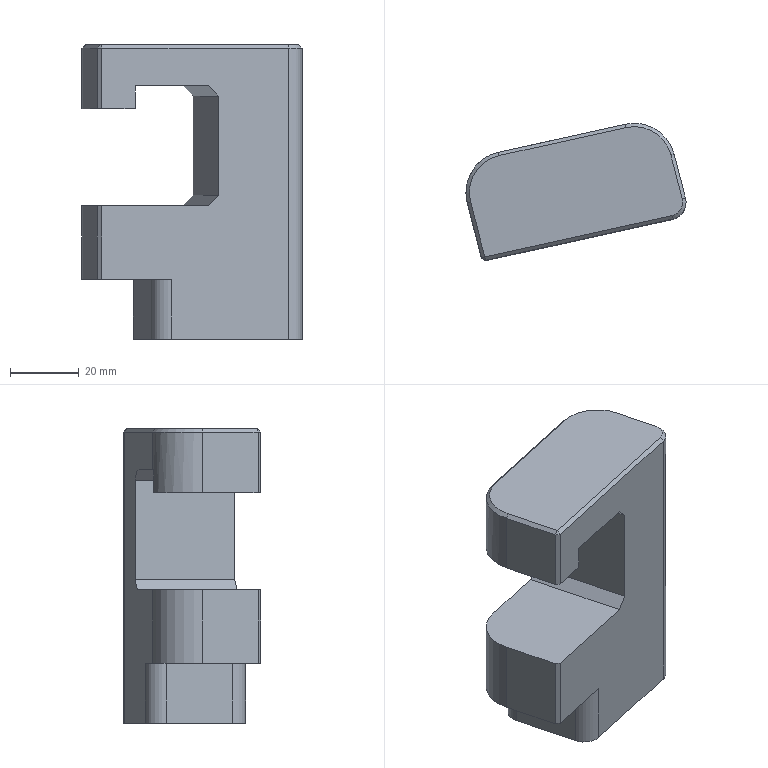Part | STEP file | 车灯-后视镜_id698_x_t | 1 solid | 40 faces | box 64.214 x 40.022 x 86 mm | volume 109388 mm3 | plane 25 | cylinder 10 | cone 5 | commonest cylinder face diameters 10 x3 24 x3 6.9 x2 8 x2
STEP:
#1=CARTESIAN_POINT('',(-118.011,95.395,72.714));
#2=VERTEX_POINT('',#1);
#3=CARTESIAN_POINT('',(-86.746,102.305,72.714));
#4=VERTEX_POINT('',#3);
#5=CARTESIAN_POINT('',(-107.9,97.63,72.714));
#6=DIRECTION('',(0.9764,0.2158,0.));
#7=VECTOR('',#6,1.);
#8=LINE('',#5,#7);
#9=EDGE_CURVE('',#2,#4,#8,.T.);
#10=ORIENTED_EDGE('',*,*,#9,.F.);
#11=CARTESIAN_POINT('',(-118.011,95.395,51.214));
#12=VERTEX_POINT('',#11);
#13=CARTESIAN_POINT('',(-118.011,95.395,51.214));
#14=DIRECTION('',(0.,0.,-1.));
#15=VECTOR('',#14,1.);
#16=LINE('',#13,#15);
#17=EDGE_CURVE('',#2,#12,#16,.T.);
#18=ORIENTED_EDGE('',*,*,#17,.T.);
#19=CARTESIAN_POINT('',(-97.663,99.892,51.214));
#20=VERTEX_POINT('',#19);
#21=CARTESIAN_POINT('',(-107.9,97.63,51.214));
#22=DIRECTION('',(-0.9764,-0.2158,0.));
#23=VECTOR('',#22,1.);
#24=LINE('',#21,#23);
#25=EDGE_CURVE('',#20,#12,#24,.T.);
#26=ORIENTED_EDGE('',*,*,#25,.F.);
#27=CARTESIAN_POINT('',(-97.663,99.892,33.714));
#28=VERTEX_POINT('',#27);
#29=CARTESIAN_POINT('',(-97.663,99.892,33.714));
#30=DIRECTION('',(0.,0.,-1.));
#31=VECTOR('',#30,1.);
#32=LINE('',#29,#31);
#33=EDGE_CURVE('',#20,#28,#32,.T.);
#34=ORIENTED_EDGE('',*,*,#33,.T.);
#35=CARTESIAN_POINT('',(-63.467,107.451,33.714));
#36=VERTEX_POINT('',#35);
#37=CARTESIAN_POINT('',(-107.9,97.63,33.714));
#38=DIRECTION('',(-0.9764,-0.2158,0.));
#39=VECTOR('',#38,1.);
#40=LINE('',#37,#39);
#41=EDGE_CURVE('',#36,#28,#40,.T.);
#42=ORIENTED_EDGE('',*,*,#41,.F.);
#43=CARTESIAN_POINT('',(-63.467,107.451,118.714));
#44=VERTEX_POINT('',#43);
#45=CARTESIAN_POINT('',(-63.467,107.451,107.714));
#46=DIRECTION('',(0.,0.,1.));
#47=VECTOR('',#46,1.);
#48=LINE('',#45,#47);
#49=EDGE_CURVE('',#36,#44,#48,.T.);
#50=ORIENTED_EDGE('',*,*,#49,.T.);
#51=CARTESIAN_POINT('',(-118.011,95.395,118.714));
#52=VERTEX_POINT('',#51);
#53=CARTESIAN_POINT('',(-107.9,97.63,118.714));
#54=DIRECTION('',(-0.9764,-0.2158,0.));
#55=VECTOR('',#54,1.);
#56=LINE('',#53,#55);
#57=EDGE_CURVE('',#44,#52,#56,.T.);
#58=ORIENTED_EDGE('',*,*,#57,.T.);
#59=CARTESIAN_POINT('',(-118.011,95.395,101.014));
#60=VERTEX_POINT('',#59);
#61=CARTESIAN_POINT('',(-118.011,95.395,101.014));
#62=DIRECTION('',(0.,0.,-1.));
#63=VECTOR('',#62,1.);
#64=LINE('',#61,#63);
#65=EDGE_CURVE('',#52,#60,#64,.T.);
#66=ORIENTED_EDGE('',*,*,#65,.T.);
#67=CARTESIAN_POINT('',(-108.24,97.554,101.014));
#68=VERTEX_POINT('',#67);
#69=CARTESIAN_POINT('',(-107.9,97.63,101.014));
#70=DIRECTION('',(0.9764,0.2158,0.));
#71=VECTOR('',#70,1.);
#72=LINE('',#69,#71);
#73=EDGE_CURVE('',#60,#68,#72,.T.);
#74=ORIENTED_EDGE('',*,*,#73,.T.);
#75=CARTESIAN_POINT('',(-108.24,97.554,107.714));
#76=VERTEX_POINT('',#75);
#77=CARTESIAN_POINT('',(-108.24,97.554,-21.603));
#78=DIRECTION('',(0.,0.,1.));
#79=VECTOR('',#78,1.);
#80=LINE('',#77,#79);
#81=EDGE_CURVE('',#68,#76,#80,.T.);
#82=ORIENTED_EDGE('',*,*,#81,.T.);
#83=CARTESIAN_POINT('',(-86.746,102.305,107.714));
#84=VERTEX_POINT('',#83);
#85=CARTESIAN_POINT('',(-107.9,97.63,107.714));
#86=DIRECTION('',(0.9764,0.2158,0.));
#87=VECTOR('',#86,1.);
#88=LINE('',#85,#87);
#89=EDGE_CURVE('',#76,#84,#88,.T.);
#90=ORIENTED_EDGE('',*,*,#89,.T.);
#91=CARTESIAN_POINT('',(-83.815,102.953,104.714));
#92=VERTEX_POINT('',#91);
#93=CARTESIAN_POINT('',(-97.329,99.966,118.547));
#94=DIRECTION('',(0.6907,0.1527,-0.7069));
#95=VECTOR('',#94,1.);
#96=LINE('',#93,#95);
#97=EDGE_CURVE('',#84,#92,#96,.T.);
#98=ORIENTED_EDGE('',*,*,#97,.T.);
#99=CARTESIAN_POINT('',(-83.815,102.953,75.714));
#100=VERTEX_POINT('',#99);
#101=CARTESIAN_POINT('',(-83.815,102.953,107.714));
#102=DIRECTION('',(0.,0.,1.));
#103=VECTOR('',#102,1.);
#104=LINE('',#101,#103);
#105=EDGE_CURVE('',#100,#92,#104,.T.);
#106=ORIENTED_EDGE('',*,*,#105,.F.);
#107=CARTESIAN_POINT('',(-80.242,103.743,79.371));
#108=DIRECTION('',(-0.6907,-0.1527,-0.7069));
#109=VECTOR('',#108,1.);
#110=LINE('',#107,#109);
#111=EDGE_CURVE('',#100,#4,#110,.T.);
#112=ORIENTED_EDGE('',*,*,#111,.T.);
#113=EDGE_LOOP('',(#10,#18,#26,#34,#42,#50,#58,#66,#74,#82,#90,#98,#106,#112));
#114=FACE_OUTER_BOUND('',#113,.T.);
#115=CARTESIAN_POINT('',(-107.9,97.63,107.714));
#116=DIRECTION('',(-0.2158,0.9764,0.));
#117=DIRECTION('',(0.,0.,1.));
#118=AXIS2_PLACEMENT_3D('',#115,#116,#117);
#119=PLANE('',#118);
#120=ADVANCED_FACE('',(#114),#119,.F.);
#121=CARTESIAN_POINT('',(-114.35,126.928,107.714));
#122=VERTEX_POINT('',#121);
#123=CARTESIAN_POINT('',(-114.35,126.928,118.714));
#124=VERTEX_POINT('',#123);
#125=CARTESIAN_POINT('',(-114.35,126.928,119.714));
#126=DIRECTION('',(0.,0.,1.));
#127=VECTOR('',#126,1.);
#128=LINE('',#125,#127);
#129=EDGE_CURVE('',#122,#124,#128,.T.);
#130=ORIENTED_EDGE('',*,*,#129,.T.);
#131=CARTESIAN_POINT('',(-77.223,135.134,118.714));
#132=VERTEX_POINT('',#131);
#133=CARTESIAN_POINT('',(-114.375,126.923,118.714));
#134=DIRECTION('',(0.9764,0.2158,0.));
#135=VECTOR('',#134,1.);
#136=LINE('',#133,#135);
#137=EDGE_CURVE('',#124,#132,#136,.T.);
#138=ORIENTED_EDGE('',*,*,#137,.T.);
#139=CARTESIAN_POINT('',(-77.223,135.134,33.714));
#140=VERTEX_POINT('',#139);
#141=CARTESIAN_POINT('',(-77.223,135.134,107.714));
#142=DIRECTION('',(0.,0.,-1.));
#143=VECTOR('',#142,1.);
#144=LINE('',#141,#143);
#145=EDGE_CURVE('',#132,#140,#144,.T.);
#146=ORIENTED_EDGE('',*,*,#145,.T.);
#147=CARTESIAN_POINT('',(-104.818,129.035,33.714));
#148=VERTEX_POINT('',#147);
#149=CARTESIAN_POINT('',(-114.375,126.923,33.714));
#150=DIRECTION('',(-0.9764,-0.2158,0.));
#151=VECTOR('',#150,1.);
#152=LINE('',#149,#151);
#153=EDGE_CURVE('',#140,#148,#152,.T.);
#154=ORIENTED_EDGE('',*,*,#153,.T.);
#155=CARTESIAN_POINT('',(-104.818,129.035,51.214));
#156=VERTEX_POINT('',#155);
#157=CARTESIAN_POINT('',(-104.818,129.035,51.214));
#158=DIRECTION('',(0.,0.,1.));
#159=VECTOR('',#158,1.);
#160=LINE('',#157,#159);
#161=EDGE_CURVE('',#148,#156,#160,.T.);
#162=ORIENTED_EDGE('',*,*,#161,.T.);
#163=CARTESIAN_POINT('',(-114.35,126.928,51.214));
#164=VERTEX_POINT('',#163);
#165=CARTESIAN_POINT('',(-114.375,126.923,51.214));
#166=DIRECTION('',(-0.9764,-0.2158,0.));
#167=VECTOR('',#166,1.);
#168=LINE('',#165,#167);
#169=EDGE_CURVE('',#156,#164,#168,.T.);
#170=ORIENTED_EDGE('',*,*,#169,.T.);
#171=CARTESIAN_POINT('',(-114.35,126.928,72.714));
#172=VERTEX_POINT('',#171);
#173=CARTESIAN_POINT('',(-114.35,126.928,72.714));
#174=DIRECTION('',(0.,0.,1.));
#175=VECTOR('',#174,1.);
#176=LINE('',#173,#175);
#177=EDGE_CURVE('',#164,#172,#176,.T.);
#178=ORIENTED_EDGE('',*,*,#177,.T.);
#179=CARTESIAN_POINT('',(-94.241,131.373,72.714));
#180=VERTEX_POINT('',#179);
#181=CARTESIAN_POINT('',(-114.375,126.923,72.714));
#182=DIRECTION('',(-0.9764,-0.2158,0.));
#183=VECTOR('',#182,1.);
#184=LINE('',#181,#183);
#185=EDGE_CURVE('',#180,#172,#184,.T.);
#186=ORIENTED_EDGE('',*,*,#185,.F.);
#187=CARTESIAN_POINT('',(-91.31,132.021,75.714));
#188=VERTEX_POINT('',#187);
#189=CARTESIAN_POINT('',(-87.226,132.923,79.894));
#190=DIRECTION('',(0.6907,0.1527,0.7069));
#191=VECTOR('',#190,1.);
#192=LINE('',#189,#191);
#193=EDGE_CURVE('',#180,#188,#192,.T.);
#194=ORIENTED_EDGE('',*,*,#193,.T.);
#195=CARTESIAN_POINT('',(-91.31,132.021,104.714));
#196=VERTEX_POINT('',#195);
#197=CARTESIAN_POINT('',(-91.31,132.021,107.714));
#198=DIRECTION('',(0.,0.,-1.));
#199=VECTOR('',#198,1.);
#200=LINE('',#197,#199);
#201=EDGE_CURVE('',#196,#188,#200,.T.);
#202=ORIENTED_EDGE('',*,*,#201,.F.);
#203=CARTESIAN_POINT('',(-94.241,131.373,107.714));
#204=VERTEX_POINT('',#203);
#205=CARTESIAN_POINT('',(-104.314,129.146,118.024));
#206=DIRECTION('',(-0.6907,-0.1527,0.7069));
#207=VECTOR('',#206,1.);
#208=LINE('',#205,#207);
#209=EDGE_CURVE('',#196,#204,#208,.T.);
#210=ORIENTED_EDGE('',*,*,#209,.T.);
#211=CARTESIAN_POINT('',(-114.375,126.923,107.714));
#212=DIRECTION('',(-0.9764,-0.2158,0.));
#213=VECTOR('',#212,1.);
#214=LINE('',#211,#213);
#215=EDGE_CURVE('',#204,#122,#214,.T.);
#216=ORIENTED_EDGE('',*,*,#215,.T.);
#217=EDGE_LOOP('',(#130,#138,#146,#154,#162,#170,#178,#186,#194,#202,#210,#216));
#218=FACE_OUTER_BOUND('',#217,.T.);
#219=CARTESIAN_POINT('',(-114.375,126.923,107.714));
#220=DIRECTION('',(-0.2158,0.9764,0.));
#221=DIRECTION('',(0.,0.,1.));
#222=AXIS2_PLACEMENT_3D('',#219,#220,#221);
#223=PLANE('',#222);
#224=ADVANCED_FACE('',(#218),#223,.T.);
#225=CARTESIAN_POINT('',(-77.008,134.158,119.714));
#226=VERTEX_POINT('',#225);
#227=CARTESIAN_POINT('',(-114.134,125.951,119.714));
#228=VERTEX_POINT('',#227);
#229=CARTESIAN_POINT('',(-114.159,125.946,119.714));
#230=DIRECTION('',(-0.9764,-0.2158,0.));
#231=VECTOR('',#230,1.);
#232=LINE('',#229,#231);
#233=EDGE_CURVE('',#226,#228,#232,.T.);
#234=ORIENTED_EDGE('',*,*,#233,.T.);
#235=CARTESIAN_POINT('',(-122.412,112.464,119.714));
#236=VERTEX_POINT('',#235);
#237=CARTESIAN_POINT('',(-111.76,115.211,119.714));
#238=DIRECTION('',(0.,0.,1.));
#239=DIRECTION('',(-1.,0.,0.));
#240=AXIS2_PLACEMENT_3D('',#237,#238,#239);
#241=CIRCLE('',#240,11.);
#242=EDGE_CURVE('',#228,#236,#241,.T.);
#243=ORIENTED_EDGE('',*,*,#242,.T.);
#244=CARTESIAN_POINT('',(-118.26,96.364,119.714));
#245=VERTEX_POINT('',#244);
#246=CARTESIAN_POINT('',(-118.019,95.429,119.714));
#247=DIRECTION('',(0.2497,-0.9683,0.));
#248=VECTOR('',#247,1.);
#249=LINE('',#246,#248);
#250=EDGE_CURVE('',#236,#245,#249,.T.);
#251=ORIENTED_EDGE('',*,*,#250,.T.);
#252=CARTESIAN_POINT('',(-63.683,108.427,119.714));
#253=VERTEX_POINT('',#252);
#254=CARTESIAN_POINT('',(-108.116,98.606,119.714));
#255=DIRECTION('',(0.9764,0.2158,0.));
#256=VECTOR('',#255,1.);
#257=LINE('',#254,#256);
#258=EDGE_CURVE('',#245,#253,#257,.T.);
#259=ORIENTED_EDGE('',*,*,#258,.T.);
#260=CARTESIAN_POINT('',(-60.673,113.332,119.714));
#261=VERTEX_POINT('',#260);
#262=CARTESIAN_POINT('',(-64.546,112.333,119.714));
#263=DIRECTION('',(0.,0.,1.));
#264=DIRECTION('',(-1.,0.,0.));
#265=AXIS2_PLACEMENT_3D('',#262,#263,#264);
#266=CIRCLE('',#265,4.);
#267=EDGE_CURVE('',#253,#261,#266,.T.);
#268=ORIENTED_EDGE('',*,*,#267,.T.);
#269=CARTESIAN_POINT('',(-63.982,126.164,119.714));
#270=VERTEX_POINT('',#269);
#271=CARTESIAN_POINT('',(-57.076,99.382,119.714));
#272=DIRECTION('',(-0.2497,0.9683,0.));
#273=VECTOR('',#272,1.);
#274=LINE('',#271,#273);
#275=EDGE_CURVE('',#261,#270,#274,.T.);
#276=ORIENTED_EDGE('',*,*,#275,.T.);
#277=CARTESIAN_POINT('',(-74.633,123.417,119.714));
#278=DIRECTION('',(0.,0.,1.));
#279=DIRECTION('',(-1.,0.,0.));
#280=AXIS2_PLACEMENT_3D('',#277,#278,#279);
#281=CIRCLE('',#280,11.);
#282=EDGE_CURVE('',#270,#226,#281,.T.);
#283=ORIENTED_EDGE('',*,*,#282,.T.);
#284=EDGE_LOOP('',(#234,#243,#251,#259,#268,#276,#283));
#285=FACE_OUTER_BOUND('',#284,.T.);
#286=CARTESIAN_POINT('',(-105.526,86.889,119.714));
#287=DIRECTION('',(0.,0.,-1.));
#288=DIRECTION('',(-0.2158,0.9764,0.));
#289=AXIS2_PLACEMENT_3D('',#286,#287,#288);
#290=PLANE('',#289);
#291=ADVANCED_FACE('',(#285),#290,.F.);
#292=ORIENTED_EDGE('',*,*,#73,.F.);
#293=CARTESIAN_POINT('',(-119.237,96.147,101.014));
#294=VERTEX_POINT('',#293);
#295=CARTESIAN_POINT('',(-119.237,96.147,101.014));
#296=DIRECTION('',(-0.8523,0.5231,0.));
#297=VECTOR('',#296,1.);
#298=LINE('',#295,#297);
#299=EDGE_CURVE('',#60,#294,#298,.T.);
#300=ORIENTED_EDGE('',*,*,#299,.T.);
#301=CARTESIAN_POINT('',(-123.38,112.214,101.014));
#302=VERTEX_POINT('',#301);
#303=CARTESIAN_POINT('',(-122.632,109.312,101.014));
#304=DIRECTION('',(0.2497,-0.9683,0.));
#305=VECTOR('',#304,1.);
#306=LINE('',#303,#305);
#307=EDGE_CURVE('',#302,#294,#306,.T.);
#308=ORIENTED_EDGE('',*,*,#307,.F.);
#309=CARTESIAN_POINT('',(-115.715,126.541,101.014));
#310=VERTEX_POINT('',#309);
#311=CARTESIAN_POINT('',(-111.76,115.211,101.014));
#312=DIRECTION('',(0.,0.,-1.));
#313=DIRECTION('',(1.,0.,0.));
#314=AXIS2_PLACEMENT_3D('',#311,#312,#313);
#315=CIRCLE('',#314,12.);
#316=EDGE_CURVE('',#302,#310,#315,.T.);
#317=ORIENTED_EDGE('',*,*,#316,.T.);
#318=CARTESIAN_POINT('',(-102.312,74.565,101.014));
#319=DIRECTION('',(0.2497,-0.9683,0.));
#320=VECTOR('',#319,1.);
#321=LINE('',#318,#320);
#322=EDGE_CURVE('',#310,#68,#321,.T.);
#323=ORIENTED_EDGE('',*,*,#322,.T.);
#324=EDGE_LOOP('',(#292,#300,#308,#317,#323));
#325=FACE_OUTER_BOUND('',#324,.T.);
#326=CARTESIAN_POINT('',(-111.137,112.276,101.014));
#327=DIRECTION('',(0.,0.,1.));
#328=DIRECTION('',(1.,0.,0.));
#329=AXIS2_PLACEMENT_3D('',#326,#327,#328);
#330=PLANE('',#329);
#331=ADVANCED_FACE('',(#325),#330,.F.);
#332=CARTESIAN_POINT('',(-123.38,112.214,72.714));
#333=VERTEX_POINT('',#332);
#334=CARTESIAN_POINT('',(-119.237,96.147,72.714));
#335=VERTEX_POINT('',#334);
#336=CARTESIAN_POINT('',(-122.449,108.604,72.714));
#337=DIRECTION('',(0.2497,-0.9683,0.));
#338=VECTOR('',#337,1.);
#339=LINE('',#336,#338);
#340=EDGE_CURVE('',#333,#335,#339,.T.);
#341=ORIENTED_EDGE('',*,*,#340,.T.);
#342=CARTESIAN_POINT('',(-107.669,89.048,72.714));
#343=DIRECTION('',(0.8523,-0.5231,0.));
#344=VECTOR('',#343,1.);
#345=LINE('',#342,#344);
#346=EDGE_CURVE('',#335,#2,#345,.T.);
#347=ORIENTED_EDGE('',*,*,#346,.T.);
#348=ORIENTED_EDGE('',*,*,#9,.T.);
#349=CARTESIAN_POINT('',(-94.215,131.271,72.714));
#350=DIRECTION('',(-0.2497,0.9683,0.));
#351=VECTOR('',#350,1.);
#352=LINE('',#349,#351);
#353=EDGE_CURVE('',#4,#180,#352,.T.);
#354=ORIENTED_EDGE('',*,*,#353,.T.);
#355=ORIENTED_EDGE('',*,*,#185,.T.);
#356=CARTESIAN_POINT('',(-111.76,115.211,72.714));
#357=DIRECTION('',(0.,0.,1.));
#358=DIRECTION('',(1.,0.,0.));
#359=AXIS2_PLACEMENT_3D('',#356,#357,#358);
#360=CIRCLE('',#359,12.);
#361=EDGE_CURVE('',#172,#333,#360,.T.);
#362=ORIENTED_EDGE('',*,*,#361,.T.);
#363=EDGE_LOOP('',(#341,#347,#348,#354,#355,#362));
#364=FACE_OUTER_BOUND('',#363,.T.);
#365=CARTESIAN_POINT('',(-90.632,116.808,72.714));
#366=DIRECTION('',(0.,0.,1.));
#367=DIRECTION('',(1.,0.,0.));
#368=AXIS2_PLACEMENT_3D('',#365,#366,#367);
#369=PLANE('',#368);
#370=ADVANCED_FACE('',(#364),#369,.T.);
#371=ORIENTED_EDGE('',*,*,#25,.T.);
#372=CARTESIAN_POINT('',(-119.237,96.147,51.214));
#373=VERTEX_POINT('',#372);
#374=CARTESIAN_POINT('',(-119.237,96.147,51.214));
#375=DIRECTION('',(-0.8523,0.5231,0.));
#376=VECTOR('',#375,1.);
#377=LINE('',#374,#376);
#378=EDGE_CURVE('',#12,#373,#377,.T.);
#379=ORIENTED_EDGE('',*,*,#378,.T.);
#380=CARTESIAN_POINT('',(-123.38,112.214,51.214));
#381=VERTEX_POINT('',#380);
#382=CARTESIAN_POINT('',(-116.144,84.151,51.214));
#383=DIRECTION('',(0.2497,-0.9683,0.));
#384=VECTOR('',#383,1.);
#385=LINE('',#382,#384);
#386=EDGE_CURVE('',#381,#373,#385,.T.);
#387=ORIENTED_EDGE('',*,*,#386,.F.);
#388=CARTESIAN_POINT('',(-111.76,115.211,51.214));
#389=DIRECTION('',(0.,0.,-1.));
#390=DIRECTION('',(-1.,0.,0.));
#391=AXIS2_PLACEMENT_3D('',#388,#389,#390);
#392=CIRCLE('',#391,12.);
#393=EDGE_CURVE('',#381,#164,#392,.T.);
#394=ORIENTED_EDGE('',*,*,#393,.T.);
#395=ORIENTED_EDGE('',*,*,#169,.F.);
#396=CARTESIAN_POINT('',(-108.581,122.904,51.214));
#397=VERTEX_POINT('',#396);
#398=CARTESIAN_POINT('',(-103.739,124.153,51.214));
#399=DIRECTION('',(0.,0.,1.));
#400=DIRECTION('',(-1.,0.,0.));
#401=AXIS2_PLACEMENT_3D('',#398,#399,#400);
#402=CIRCLE('',#401,5.);
#403=EDGE_CURVE('',#156,#397,#402,.T.);
#404=ORIENTED_EDGE('',*,*,#403,.T.);
#405=CARTESIAN_POINT('',(-103.584,103.526,51.214));
#406=VERTEX_POINT('',#405);
#407=CARTESIAN_POINT('',(-99.682,88.396,51.214));
#408=DIRECTION('',(0.2497,-0.9683,0.));
#409=VECTOR('',#408,1.);
#410=LINE('',#407,#409);
#411=EDGE_CURVE('',#397,#406,#410,.T.);
#412=ORIENTED_EDGE('',*,*,#411,.T.);
#413=CARTESIAN_POINT('',(-98.742,104.774,51.214));
#414=DIRECTION('',(0.,0.,1.));
#415=DIRECTION('',(-1.,0.,0.));
#416=AXIS2_PLACEMENT_3D('',#413,#414,#415);
#417=CIRCLE('',#416,5.);
#418=EDGE_CURVE('',#406,#20,#417,.T.);
#419=ORIENTED_EDGE('',*,*,#418,.T.);
#420=EDGE_LOOP('',(#371,#379,#387,#394,#395,#404,#412,#419));
#421=FACE_OUTER_BOUND('',#420,.T.);
#422=CARTESIAN_POINT('',(-105.526,86.889,51.214));
#423=DIRECTION('',(0.,0.,-1.));
#424=DIRECTION('',(-0.2158,0.9764,0.));
#425=AXIS2_PLACEMENT_3D('',#422,#423,#424);
#426=PLANE('',#425);
#427=ADVANCED_FACE('',(#421),#426,.T.);
#428=ORIENTED_EDGE('',*,*,#215,.F.);
#429=CARTESIAN_POINT('',(-90.677,117.552,107.714));
#430=DIRECTION('',(0.2497,-0.9683,0.));
#431=VECTOR('',#430,1.);
#432=LINE('',#429,#431);
#433=EDGE_CURVE('',#204,#84,#432,.T.);
#434=ORIENTED_EDGE('',*,*,#433,.T.);
#435=ORIENTED_EDGE('',*,*,#89,.F.);
#436=CARTESIAN_POINT('',(-115.715,126.541,107.714));
#437=VERTEX_POINT('',#436);
#438=CARTESIAN_POINT('',(-102.312,74.565,107.714));
#439=DIRECTION('',(0.2497,-0.9683,0.));
#440=VECTOR('',#439,1.);
#441=LINE('',#438,#440);
#442=EDGE_CURVE('',#437,#76,#441,.T.);
#443=ORIENTED_EDGE('',*,*,#442,.F.);
#444=CARTESIAN_POINT('',(-111.76,115.211,107.714));
#445=DIRECTION('',(0.,0.,-1.));
#446=DIRECTION('',(1.,0.,0.));
#447=AXIS2_PLACEMENT_3D('',#444,#445,#446);
#448=CIRCLE('',#447,12.);
#449=EDGE_CURVE('',#437,#122,#448,.T.);
#450=ORIENTED_EDGE('',*,*,#449,.T.);
#451=EDGE_LOOP('',(#428,#434,#435,#443,#450));
#452=FACE_OUTER_BOUND('',#451,.T.);
#453=CARTESIAN_POINT('',(-111.137,112.276,107.714));
#454=DIRECTION('',(0.,0.,1.));
#455=DIRECTION('',(1.,0.,0.));
#456=AXIS2_PLACEMENT_3D('',#453,#454,#455);
#457=PLANE('',#456);
#458=ADVANCED_FACE('',(#452),#457,.F.);
#459=ORIENTED_EDGE('',*,*,#105,.T.);
#460=CARTESIAN_POINT('',(-85.156,108.157,104.714));
#461=DIRECTION('',(-0.2497,0.9683,0.));
#462=VECTOR('',#461,1.);
#463=LINE('',#460,#462);
#464=EDGE_CURVE('',#92,#196,#463,.T.);
#465=ORIENTED_EDGE('',*,*,#464,.T.);
#466=ORIENTED_EDGE('',*,*,#201,.T.);
#467=CARTESIAN_POINT('',(-83.815,102.953,75.714));
#468=DIRECTION('',(0.2497,-0.9683,0.));
#469=VECTOR('',#468,1.);
#470=LINE('',#467,#469);
#471=EDGE_CURVE('',#188,#100,#470,.T.);
#472=ORIENTED_EDGE('',*,*,#471,.T.);
#473=EDGE_LOOP('',(#459,#465,#466,#472));
#474=FACE_OUTER_BOUND('',#473,.T.);
#475=CARTESIAN_POINT('',(-85.156,108.157,96.214));
#476=DIRECTION('',(-0.9683,-0.2497,0.));
#477=DIRECTION('',(0.2497,-0.9683,0.));
#478=AXIS2_PLACEMENT_3D('',#475,#476,#477);
#479=PLANE('',#478);
#480=ADVANCED_FACE('',(#474),#479,.T.);
#481=ORIENTED_EDGE('',*,*,#322,.F.);
#482=CARTESIAN_POINT('',(-115.715,126.541,101.014));
#483=DIRECTION('',(0.,0.,1.));
#484=VECTOR('',#483,1.);
#485=LINE('',#482,#484);
#486=EDGE_CURVE('',#310,#437,#485,.T.);
#487=ORIENTED_EDGE('',*,*,#486,.T.);
#488=ORIENTED_EDGE('',*,*,#442,.T.);
#489=ORIENTED_EDGE('',*,*,#81,.F.);
#490=EDGE_LOOP('',(#481,#487,#488,#489));
#491=FACE_OUTER_BOUND('',#490,.T.);
#492=CARTESIAN_POINT('',(-102.312,74.565,-21.603));
#493=DIRECTION('',(0.9683,0.2497,0.));
#494=DIRECTION('',(-0.2497,0.9683,0.));
#495=AXIS2_PLACEMENT_3D('',#492,#493,#494);
#496=PLANE('',#495);
#497=ADVANCED_FACE('',(#491),#496,.T.);
#498=CARTESIAN_POINT('',(-76.08,120.909,33.714));
#499=VERTEX_POINT('',#498);
#500=CARTESIAN_POINT('',(-72.08,120.909,33.714));
#501=DIRECTION('',(0.,0.,-1.));
#502=DIRECTION('',(-1.,0.,0.));
#503=AXIS2_PLACEMENT_3D('',#500,#501,#502);
#504=CIRCLE('',#503,4.);
#505=EDGE_CURVE('',#499,#499,#504,.T.);
#506=ORIENTED_EDGE('',*,*,#505,.F.);
#507=EDGE_LOOP('',(#506));
#508=FACE_BOUND('',#507,.T.);
#509=CARTESIAN_POINT('',(-100.396,114.65,33.714));
#510=VERTEX_POINT('',#509);
#511=CARTESIAN_POINT('',(-96.491,115.513,33.714));
#512=DIRECTION('',(0.,0.,-1.));
#513=DIRECTION('',(-0.9764,-0.2158,0.));
#514=AXIS2_PLACEMENT_3D('',#511,#512,#513);
#515=CIRCLE('',#514,4.);
#516=EDGE_CURVE('',#510,#510,#515,.T.);
#517=ORIENTED_EDGE('',*,*,#516,.F.);
#518=EDGE_LOOP('',(#517));
#519=FACE_BOUND('',#518,.T.);
#520=CARTESIAN_POINT('',(-108.581,122.904,33.714));
#521=VERTEX_POINT('',#520);
#522=CARTESIAN_POINT('',(-103.584,103.526,33.714));
#523=VERTEX_POINT('',#522);
#524=CARTESIAN_POINT('',(-99.682,88.396,33.714));
#525=DIRECTION('',(0.2497,-0.9683,0.));
#526=VECTOR('',#525,1.);
#527=LINE('',#524,#526);
#528=EDGE_CURVE('',#521,#523,#527,.T.);
#529=ORIENTED_EDGE('',*,*,#528,.F.);
#530=CARTESIAN_POINT('',(-103.739,124.153,33.714));
#531=DIRECTION('',(0.,0.,-1.));
#532=DIRECTION('',(-1.,0.,0.));
#533=AXIS2_PLACEMENT_3D('',#530,#531,#532);
#534=CIRCLE('',#533,5.);
#535=EDGE_CURVE('',#521,#148,#534,.T.);
#536=ORIENTED_EDGE('',*,*,#535,.T.);
#537=ORIENTED_EDGE('',*,*,#153,.F.);
#538=CARTESIAN_POINT('',(-63.014,126.413,33.714));
#539=VERTEX_POINT('',#538);
#540=CARTESIAN_POINT('',(-74.633,123.417,33.714));
#541=DIRECTION('',(0.,0.,-1.));
#542=DIRECTION('',(-1.,0.,0.));
#543=AXIS2_PLACEMENT_3D('',#540,#541,#542);
#544=CIRCLE('',#543,12.);
#545=EDGE_CURVE('',#140,#539,#544,.T.);
#546=ORIENTED_EDGE('',*,*,#545,.T.);
#547=CARTESIAN_POINT('',(-59.705,113.581,33.714));
#548=VERTEX_POINT('',#547);
#549=CARTESIAN_POINT('',(-56.108,99.632,33.714));
#550=DIRECTION('',(0.2497,-0.9683,0.));
#551=VECTOR('',#550,1.);
#552=LINE('',#549,#551);
#553=EDGE_CURVE('',#539,#548,#552,.T.);
#554=ORIENTED_EDGE('',*,*,#553,.T.);
#555=CARTESIAN_POINT('',(-64.546,112.333,33.714));
#556=DIRECTION('',(0.,0.,-1.));
#557=DIRECTION('',(-1.,0.,0.));
#558=AXIS2_PLACEMENT_3D('',#555,#556,#557);
#559=CIRCLE('',#558,5.);
#560=EDGE_CURVE('',#548,#36,#559,.T.);
#561=ORIENTED_EDGE('',*,*,#560,.T.);
#562=ORIENTED_EDGE('',*,*,#41,.T.);
#563=CARTESIAN_POINT('',(-98.742,104.774,33.714));
#564=DIRECTION('',(0.,0.,-1.));
#565=DIRECTION('',(-1.,0.,0.));
#566=AXIS2_PLACEMENT_3D('',#563,#564,#565);
#567=CIRCLE('',#566,5.);
#568=EDGE_CURVE('',#28,#523,#567,.T.);
#569=ORIENTED_EDGE('',*,*,#568,.T.);
#570=EDGE_LOOP('',(#529,#536,#537,#546,#554,#561,#562,#569));
#571=FACE_BOUND('',#570,.T.);
#572=CARTESIAN_POINT('',(-105.526,86.889,33.714));
#573=DIRECTION('',(0.,0.,-1.));
#574=DIRECTION('',(-0.2158,0.9764,0.));
#575=AXIS2_PLACEMENT_3D('',#572,#573,#574);
#576=PLANE('',#575);
#577=ADVANCED_FACE('',(#508,#519,#571),#576,.T.);
#578=ORIENTED_EDGE('',*,*,#411,.F.);
#579=CARTESIAN_POINT('',(-108.581,122.904,33.714));
#580=DIRECTION('',(0.,0.,-1.));
#581=VECTOR('',#580,1.);
#582=LINE('',#579,#581);
#583=EDGE_CURVE('',#397,#521,#582,.T.);
#584=ORIENTED_EDGE('',*,*,#583,.T.);
#585=ORIENTED_EDGE('',*,*,#528,.T.);
#586=CARTESIAN_POINT('',(-103.584,103.526,51.214));
#587=DIRECTION('',(0.,0.,1.));
#588=VECTOR('',#587,1.);
#589=LINE('',#586,#588);
#590=EDGE_CURVE('',#523,#406,#589,.T.);
#591=ORIENTED_EDGE('',*,*,#590,.T.);
#592=EDGE_LOOP('',(#578,#584,#585,#591));
#593=FACE_OUTER_BOUND('',#592,.T.);
#594=CARTESIAN_POINT('',(-96.502,76.063,-21.603));
#595=DIRECTION('',(0.9683,0.2497,0.));
#596=DIRECTION('',(-0.2497,0.9683,0.));
#597=AXIS2_PLACEMENT_3D('',#594,#595,#596);
#598=PLANE('',#597);
#599=ADVANCED_FACE('',(#593),#598,.F.);
#600=CARTESIAN_POINT('',(-93.122,116.258,51.714));
#601=VERTEX_POINT('',#600);
#602=CARTESIAN_POINT('',(-96.491,115.513,51.714));
#603=DIRECTION('',(0.,0.,1.));
#604=DIRECTION('',(0.9764,0.2158,0.));
#605=AXIS2_PLACEMENT_3D('',#602,#603,#604);
#606=CIRCLE('',#605,3.45);
#607=EDGE_CURVE('',#601,#601,#606,.T.);
#608=ORIENTED_EDGE('',*,*,#607,.T.);
#609=EDGE_LOOP('',(#608));
#610=FACE_BOUND('',#609,.T.);
#611=CARTESIAN_POINT('',(-99.859,114.769,49.714));
#612=VERTEX_POINT('',#611);
#613=CARTESIAN_POINT('',(-96.491,115.513,49.714));
#614=DIRECTION('',(0.,0.,1.));
#615=DIRECTION('',(-0.9764,-0.2158,0.));
#616=AXIS2_PLACEMENT_3D('',#613,#614,#615);
#617=CIRCLE('',#616,3.45);
#618=EDGE_CURVE('',#612,#612,#617,.T.);
#619=ORIENTED_EDGE('',*,*,#618,.F.);
#620=EDGE_LOOP('',(#619));
#621=FACE_BOUND('',#620,.T.);
#622=CARTESIAN_POINT('',(-96.491,115.513,49.714));
#623=DIRECTION('',(0.,0.,1.));
#624=DIRECTION('',(-0.9764,-0.2158,0.));
#625=AXIS2_PLACEMENT_3D('',#622,#623,#624);
#626=CYLINDRICAL_SURFACE('',#625,3.45);
#627=ADVANCED_FACE('',(#610,#621),#626,.F.);
#628=ORIENTED_EDGE('',*,*,#607,.F.);
#629=EDGE_LOOP('',(#628));
#630=FACE_BOUND('',#629,.T.);
#631=CARTESIAN_POINT('',(-96.491,115.513,53.787));
#632=VERTEX_POINT('',#631);
#633=VERTEX_LOOP('',#632);
#634=FACE_BOUND('',#633,.T.);
#635=CARTESIAN_POINT('',(-96.491,115.513,53.787));
#636=DIRECTION('',(0.,0.,-1.));
#637=DIRECTION('',(0.9764,0.2158,0.));
#638=AXIS2_PLACEMENT_3D('',#635,#636,#637);
#639=CONICAL_SURFACE('',#638,0.,59.);
#640=ADVANCED_FACE('',(#630,#634),#639,.F.);
#641=ORIENTED_EDGE('',*,*,#618,.T.);
#642=EDGE_LOOP('',(#641));
#643=FACE_BOUND('',#642,.T.);
#644=CARTESIAN_POINT('',(-92.585,116.377,49.714));
#645=VERTEX_POINT('',#644);
#646=CARTESIAN_POINT('',(-96.491,115.513,49.714));
#647=DIRECTION('',(0.,0.,1.));
#648=DIRECTION('',(0.9764,0.2158,0.));
#649=AXIS2_PLACEMENT_3D('',#646,#647,#648);
#650=CIRCLE('',#649,4.);
#651=EDGE_CURVE('',#645,#645,#650,.T.);
#652=ORIENTED_EDGE('',*,*,#651,.F.);
#653=EDGE_LOOP('',(#652));
#654=FACE_BOUND('',#653,.T.);
#655=CARTESIAN_POINT('',(-96.491,115.513,49.714));
#656=DIRECTION('',(0.,0.,1.));
#657=DIRECTION('',(-0.9764,-0.2158,0.));
#658=AXIS2_PLACEMENT_3D('',#655,#656,#657);
#659=PLANE('',#658);
#660=ADVANCED_FACE('',(#643,#654),#659,.F.);
#661=ORIENTED_EDGE('',*,*,#651,.T.);
#662=EDGE_LOOP('',(#661));
#663=FACE_BOUND('',#662,.T.);
#664=ORIENTED_EDGE('',*,*,#516,.T.);
#665=EDGE_LOOP('',(#664));
#666=FACE_BOUND('',#665,.T.);
#667=CARTESIAN_POINT('',(-96.491,115.513,33.714));
#668=DIRECTION('',(0.,0.,1.));
#669=DIRECTION('',(-0.9764,-0.2158,0.));
#670=AXIS2_PLACEMENT_3D('',#667,#668,#669);
#671=CYLINDRICAL_SURFACE('',#670,4.);
#672=ADVANCED_FACE('',(#663,#666),#671,.F.);
#673=CARTESIAN_POINT('',(-68.711,121.654,51.714));
#674=VERTEX_POINT('',#673);
#675=CARTESIAN_POINT('',(-72.08,120.909,51.714));
#676=DIRECTION('',(0.,0.,1.));
#677=DIRECTION('',(0.9764,0.2158,0.));
#678=AXIS2_PLACEMENT_3D('',#675,#676,#677);
#679=CIRCLE('',#678,3.45);
#680=EDGE_CURVE('',#674,#674,#679,.T.);
#681=ORIENTED_EDGE('',*,*,#680,.T.);
#682=EDGE_LOOP('',(#681));
#683=FACE_BOUND('',#682,.T.);
#684=CARTESIAN_POINT('',(-75.449,120.164,49.714));
#685=VERTEX_POINT('',#684);
#686=CARTESIAN_POINT('',(-72.08,120.909,49.714));
#687=DIRECTION('',(0.,0.,1.));
#688=DIRECTION('',(-0.9764,-0.2158,0.));
#689=AXIS2_PLACEMENT_3D('',#686,#687,#688);
#690=CIRCLE('',#689,3.45);
#691=EDGE_CURVE('',#685,#685,#690,.T.);
#692=ORIENTED_EDGE('',*,*,#691,.F.);
#693=EDGE_LOOP('',(#692));
#694=FACE_BOUND('',#693,.T.);
#695=CARTESIAN_POINT('',(-72.08,120.909,49.714));
#696=DIRECTION('',(0.,0.,1.));
#697=DIRECTION('',(-0.9764,-0.2158,0.));
#698=AXIS2_PLACEMENT_3D('',#695,#696,#697);
#699=CYLINDRICAL_SURFACE('',#698,3.45);
#700=ADVANCED_FACE('',(#683,#694),#699,.F.);
#701=ORIENTED_EDGE('',*,*,#680,.F.);
#702=EDGE_LOOP('',(#701));
#703=FACE_BOUND('',#702,.T.);
#704=CARTESIAN_POINT('',(-72.08,120.909,53.787));
#705=VERTEX_POINT('',#704);
#706=VERTEX_LOOP('',#705);
#707=FACE_BOUND('',#706,.T.);
#708=CARTESIAN_POINT('',(-72.08,120.909,53.787));
#709=DIRECTION('',(0.,0.,-1.));
#710=DIRECTION('',(0.9764,0.2158,0.));
#711=AXIS2_PLACEMENT_3D('',#708,#709,#710);
#712=CONICAL_SURFACE('',#711,0.,59.);
#713=ADVANCED_FACE('',(#703,#707),#712,.F.);
#714=ORIENTED_EDGE('',*,*,#691,.T.);
#715=EDGE_LOOP('',(#714));
#716=FACE_BOUND('',#715,.T.);
#717=CARTESIAN_POINT('',(-68.174,121.772,49.714));
#718=VERTEX_POINT('',#717);
#719=CARTESIAN_POINT('',(-72.08,120.909,49.714));
#720=DIRECTION('',(0.,0.,1.));
#721=DIRECTION('',(0.9764,0.2158,0.));
#722=AXIS2_PLACEMENT_3D('',#719,#720,#721);
#723=CIRCLE('',#722,4.);
#724=EDGE_CURVE('',#718,#718,#723,.T.);
#725=ORIENTED_EDGE('',*,*,#724,.F.);
#726=EDGE_LOOP('',(#725));
#727=FACE_BOUND('',#726,.T.);
#728=CARTESIAN_POINT('',(-72.08,120.909,49.714));
#729=DIRECTION('',(0.,0.,1.));
#730=DIRECTION('',(-0.9764,-0.2158,0.));
#731=AXIS2_PLACEMENT_3D('',#728,#729,#730);
#732=PLANE('',#731);
#733=ADVANCED_FACE('',(#716,#727),#732,.F.);
#734=ORIENTED_EDGE('',*,*,#724,.T.);
#735=EDGE_LOOP('',(#734));
#736=FACE_BOUND('',#735,.T.);
#737=ORIENTED_EDGE('',*,*,#505,.T.);
#738=EDGE_LOOP('',(#737));
#739=FACE_BOUND('',#738,.T.);
#740=CARTESIAN_POINT('',(-72.08,120.909,33.714));
#741=DIRECTION('',(0.,0.,1.));
#742=DIRECTION('',(-0.9764,-0.2158,0.));
#743=AXIS2_PLACEMENT_3D('',#740,#741,#742);
#744=CYLINDRICAL_SURFACE('',#743,4.);
#745=ADVANCED_FACE('',(#736,#739),#744,.F.);
#746=ORIENTED_EDGE('',*,*,#386,.T.);
#747=CARTESIAN_POINT('',(-119.237,96.147,72.714));
#748=DIRECTION('',(0.,0.,1.));
#749=VECTOR('',#748,1.);
#750=LINE('',#747,#749);
#751=EDGE_CURVE('',#373,#335,#750,.T.);
#752=ORIENTED_EDGE('',*,*,#751,.T.);
#753=ORIENTED_EDGE('',*,*,#340,.F.);
#754=CARTESIAN_POINT('',(-123.38,112.214,51.214));
#755=DIRECTION('',(0.,0.,-1.));
#756=VECTOR('',#755,1.);
#757=LINE('',#754,#756);
#758=EDGE_CURVE('',#333,#381,#757,.T.);
#759=ORIENTED_EDGE('',*,*,#758,.T.);
#760=EDGE_LOOP('',(#746,#752,#753,#759));
#761=FACE_OUTER_BOUND('',#760,.T.);
#762=CARTESIAN_POINT('',(-119.889,98.675,96.214));
#763=DIRECTION('',(-0.9683,-0.2497,0.));
#764=DIRECTION('',(0.2497,-0.9683,0.));
#765=AXIS2_PLACEMENT_3D('',#762,#763,#764);
#766=PLANE('',#765);
#767=ADVANCED_FACE('',(#761),#766,.T.);
#768=ORIENTED_EDGE('',*,*,#307,.T.);
#769=CARTESIAN_POINT('',(-119.237,96.147,118.714));
#770=VERTEX_POINT('',#769);
#771=CARTESIAN_POINT('',(-119.237,96.147,119.714));
#772=DIRECTION('',(0.,0.,1.));
#773=VECTOR('',#772,1.);
#774=LINE('',#771,#773);
#775=EDGE_CURVE('',#294,#770,#774,.T.);
#776=ORIENTED_EDGE('',*,*,#775,.T.);
#777=CARTESIAN_POINT('',(-123.38,112.214,118.714));
#778=VERTEX_POINT('',#777);
#779=CARTESIAN_POINT('',(-123.38,112.214,118.714));
#780=DIRECTION('',(-0.2497,0.9683,0.));
#781=VECTOR('',#780,1.);
#782=LINE('',#779,#781);
#783=EDGE_CURVE('',#770,#778,#782,.T.);
#784=ORIENTED_EDGE('',*,*,#783,.T.);
#785=CARTESIAN_POINT('',(-123.38,112.214,101.014));
#786=DIRECTION('',(0.,0.,-1.));
#787=VECTOR('',#786,1.);
#788=LINE('',#785,#787);
#789=EDGE_CURVE('',#778,#302,#788,.T.);
#790=ORIENTED_EDGE('',*,*,#789,.T.);
#791=EDGE_LOOP('',(#768,#776,#784,#790));
#792=FACE_OUTER_BOUND('',#791,.T.);
#793=CARTESIAN_POINT('',(-119.889,98.675,96.214));
#794=DIRECTION('',(-0.9683,-0.2497,0.));
#795=DIRECTION('',(0.2497,-0.9683,0.));
#796=AXIS2_PLACEMENT_3D('',#793,#794,#795);
#797=PLANE('',#796);
#798=ADVANCED_FACE('',(#792),#797,.T.);
#799=CARTESIAN_POINT('',(-63.014,126.413,118.714));
#800=VERTEX_POINT('',#799);
#801=CARTESIAN_POINT('',(-63.014,126.413,61.964));
#802=DIRECTION('',(0.,0.,1.));
#803=VECTOR('',#802,1.);
#804=LINE('',#801,#803);
#805=EDGE_CURVE('',#539,#800,#804,.T.);
#806=ORIENTED_EDGE('',*,*,#805,.T.);
#807=CARTESIAN_POINT('',(-59.705,113.581,118.714));
#808=VERTEX_POINT('',#807);
#809=CARTESIAN_POINT('',(-62.699,125.194,118.714));
#810=DIRECTION('',(0.2497,-0.9683,0.));
#811=VECTOR('',#810,1.);
#812=LINE('',#809,#811);
#813=EDGE_CURVE('',#800,#808,#812,.T.);
#814=ORIENTED_EDGE('',*,*,#813,.T.);
#815=CARTESIAN_POINT('',(-59.705,113.581,61.964));
#816=DIRECTION('',(0.,0.,-1.));
#817=VECTOR('',#816,1.);
#818=LINE('',#815,#817);
#819=EDGE_CURVE('',#808,#548,#818,.T.);
#820=ORIENTED_EDGE('',*,*,#819,.T.);
#821=ORIENTED_EDGE('',*,*,#553,.F.);
#822=EDGE_LOOP('',(#806,#814,#820,#821));
#823=FACE_OUTER_BOUND('',#822,.T.);
#824=CARTESIAN_POINT('',(-62.699,125.194,61.964));
#825=DIRECTION('',(-0.9683,-0.2497,0.));
#826=DIRECTION('',(0.2497,-0.9683,0.));
#827=AXIS2_PLACEMENT_3D('',#824,#825,#826);
#828=PLANE('',#827);
#829=ADVANCED_FACE('',(#823),#828,.F.);
#830=ORIENTED_EDGE('',*,*,#145,.F.);
#831=CARTESIAN_POINT('',(-74.633,123.417,118.714));
#832=DIRECTION('',(0.,0.,-1.));
#833=DIRECTION('',(-1.,0.,0.));
#834=AXIS2_PLACEMENT_3D('',#831,#832,#833);
#835=CIRCLE('',#834,12.);
#836=EDGE_CURVE('',#132,#800,#835,.T.);
#837=ORIENTED_EDGE('',*,*,#836,.T.);
#838=ORIENTED_EDGE('',*,*,#805,.F.);
#839=ORIENTED_EDGE('',*,*,#545,.F.);
#840=EDGE_LOOP('',(#830,#837,#838,#839));
#841=FACE_OUTER_BOUND('',#840,.T.);
#842=CARTESIAN_POINT('',(-74.633,123.417,107.714));
#843=DIRECTION('',(0.,0.,1.));
#844=DIRECTION('',(1.,0.,0.));
#845=AXIS2_PLACEMENT_3D('',#842,#843,#844);
#846=CYLINDRICAL_SURFACE('',#845,12.);
#847=ADVANCED_FACE('',(#841),#846,.T.);
#848=ORIENTED_EDGE('',*,*,#403,.F.);
#849=ORIENTED_EDGE('',*,*,#161,.F.);
#850=ORIENTED_EDGE('',*,*,#535,.F.);
#851=ORIENTED_EDGE('',*,*,#583,.F.);
#852=EDGE_LOOP('',(#848,#849,#850,#851));
#853=FACE_OUTER_BOUND('',#852,.T.);
#854=CARTESIAN_POINT('',(-103.739,124.153,-21.603));
#855=DIRECTION('',(0.,0.,1.));
#856=DIRECTION('',(1.,0.,0.));
#857=AXIS2_PLACEMENT_3D('',#854,#855,#856);
#858=CYLINDRICAL_SURFACE('',#857,5.);
#859=ADVANCED_FACE('',(#853),#858,.T.);
#860=ORIENTED_EDGE('',*,*,#418,.F.);
#861=ORIENTED_EDGE('',*,*,#590,.F.);
#862=ORIENTED_EDGE('',*,*,#568,.F.);
#863=ORIENTED_EDGE('',*,*,#33,.F.);
#864=EDGE_LOOP('',(#860,#861,#862,#863));
#865=FACE_OUTER_BOUND('',#864,.T.);
#866=CARTESIAN_POINT('',(-98.742,104.774,107.714));
#867=DIRECTION('',(0.,0.,-1.));
#868=DIRECTION('',(-1.,0.,0.));
#869=AXIS2_PLACEMENT_3D('',#866,#867,#868);
#870=CYLINDRICAL_SURFACE('',#869,5.);
#871=ADVANCED_FACE('',(#865),#870,.T.);
#872=ORIENTED_EDGE('',*,*,#819,.F.);
#873=CARTESIAN_POINT('',(-64.546,112.333,118.714));
#874=DIRECTION('',(0.,0.,-1.));
#875=DIRECTION('',(-1.,0.,0.));
#876=AXIS2_PLACEMENT_3D('',#873,#874,#875);
#877=CIRCLE('',#876,5.);
#878=EDGE_CURVE('',#808,#44,#877,.T.);
#879=ORIENTED_EDGE('',*,*,#878,.T.);
#880=ORIENTED_EDGE('',*,*,#49,.F.);
#881=ORIENTED_EDGE('',*,*,#560,.F.);
#882=EDGE_LOOP('',(#872,#879,#880,#881));
#883=FACE_OUTER_BOUND('',#882,.T.);
#884=CARTESIAN_POINT('',(-64.546,112.333,107.714));
#885=DIRECTION('',(0.,0.,1.));
#886=DIRECTION('',(1.,0.,0.));
#887=AXIS2_PLACEMENT_3D('',#884,#885,#886);
#888=CYLINDRICAL_SURFACE('',#887,5.);
#889=ADVANCED_FACE('',(#883),#888,.T.);
#890=ORIENTED_EDGE('',*,*,#789,.F.);
#891=CARTESIAN_POINT('',(-111.76,115.211,118.714));
#892=DIRECTION('',(0.,0.,-1.));
#893=DIRECTION('',(-1.,0.,0.));
#894=AXIS2_PLACEMENT_3D('',#891,#892,#893);
#895=CIRCLE('',#894,12.);
#896=EDGE_CURVE('',#778,#124,#895,.T.);
#897=ORIENTED_EDGE('',*,*,#896,.T.);
#898=ORIENTED_EDGE('',*,*,#129,.F.);
#899=ORIENTED_EDGE('',*,*,#449,.F.);
#900=ORIENTED_EDGE('',*,*,#486,.F.);
#901=ORIENTED_EDGE('',*,*,#316,.F.);
#902=EDGE_LOOP('',(#890,#897,#898,#899,#900,#901));
#903=FACE_OUTER_BOUND('',#902,.T.);
#904=CARTESIAN_POINT('',(-111.76,115.211,96.214));
#905=DIRECTION('',(0.,0.,-1.));
#906=DIRECTION('',(-1.,0.,0.));
#907=AXIS2_PLACEMENT_3D('',#904,#905,#906);
#908=CYLINDRICAL_SURFACE('',#907,12.);
#909=ADVANCED_FACE('',(#903),#908,.T.);
#910=ORIENTED_EDGE('',*,*,#361,.F.);
#911=ORIENTED_EDGE('',*,*,#177,.F.);
#912=ORIENTED_EDGE('',*,*,#393,.F.);
#913=ORIENTED_EDGE('',*,*,#758,.F.);
#914=EDGE_LOOP('',(#910,#911,#912,#913));
#915=FACE_OUTER_BOUND('',#914,.T.);
#916=CARTESIAN_POINT('',(-111.76,115.211,96.214));
#917=DIRECTION('',(0.,0.,-1.));
#918=DIRECTION('',(-1.,0.,0.));
#919=AXIS2_PLACEMENT_3D('',#916,#917,#918);
#920=CYLINDRICAL_SURFACE('',#919,12.);
#921=ADVANCED_FACE('',(#915),#920,.T.);
#922=ORIENTED_EDGE('',*,*,#209,.F.);
#923=ORIENTED_EDGE('',*,*,#464,.F.);
#924=ORIENTED_EDGE('',*,*,#97,.F.);
#925=ORIENTED_EDGE('',*,*,#433,.F.);
#926=EDGE_LOOP('',(#922,#923,#924,#925));
#927=FACE_OUTER_BOUND('',#926,.T.);
#928=CARTESIAN_POINT('',(-90.677,117.552,107.714));
#929=DIRECTION('',(0.6847,0.1766,0.7071));
#930=DIRECTION('',(0.7184,0.,-0.6956));
#931=AXIS2_PLACEMENT_3D('',#928,#929,#930);
#932=PLANE('',#931);
#933=ADVANCED_FACE('',(#927),#932,.F.);
#934=ORIENTED_EDGE('',*,*,#193,.F.);
#935=ORIENTED_EDGE('',*,*,#353,.F.);
#936=ORIENTED_EDGE('',*,*,#111,.F.);
#937=ORIENTED_EDGE('',*,*,#471,.F.);
#938=EDGE_LOOP('',(#934,#935,#936,#937));
#939=FACE_OUTER_BOUND('',#938,.T.);
#940=CARTESIAN_POINT('',(-85.156,108.157,75.714));
#941=DIRECTION('',(-0.6847,-0.1766,0.7071));
#942=DIRECTION('',(0.7184,0.,0.6956));
#943=AXIS2_PLACEMENT_3D('',#940,#941,#942);
#944=PLANE('',#943);
#945=ADVANCED_FACE('',(#939),#944,.T.);
#946=ORIENTED_EDGE('',*,*,#378,.F.);
#947=ORIENTED_EDGE('',*,*,#17,.F.);
#948=ORIENTED_EDGE('',*,*,#346,.F.);
#949=ORIENTED_EDGE('',*,*,#751,.F.);
#950=EDGE_LOOP('',(#946,#947,#948,#949));
#951=FACE_OUTER_BOUND('',#950,.T.);
#952=CARTESIAN_POINT('',(-119.237,96.147,96.214));
#953=DIRECTION('',(-0.5231,-0.8523,0.));
#954=DIRECTION('',(0.8523,-0.5231,0.));
#955=AXIS2_PLACEMENT_3D('',#952,#953,#954);
#956=PLANE('',#955);
#957=ADVANCED_FACE('',(#951),#956,.T.);
#958=CARTESIAN_POINT('',(-63.014,126.413,118.714));
#959=DIRECTION('',(-0.6847,-0.1766,0.7071));
#960=VECTOR('',#959,1.);
#961=LINE('',#958,#960);
#962=EDGE_CURVE('',#800,#270,#961,.T.);
#963=ORIENTED_EDGE('',*,*,#962,.F.);
#964=ORIENTED_EDGE('',*,*,#836,.F.);
#965=CARTESIAN_POINT('',(-77.008,134.158,119.714));
#966=DIRECTION('',(-0.1526,0.6904,-0.7071));
#967=VECTOR('',#966,1.);
#968=LINE('',#965,#967);
#969=EDGE_CURVE('',#226,#132,#968,.T.);
#970=ORIENTED_EDGE('',*,*,#969,.F.);
#971=ORIENTED_EDGE('',*,*,#282,.F.);
#972=EDGE_LOOP('',(#963,#964,#970,#971));
#973=FACE_OUTER_BOUND('',#972,.T.);
#974=CARTESIAN_POINT('',(-74.633,123.417,119.714));
#975=DIRECTION('',(0.,0.,-1.));
#976=DIRECTION('',(-1.,0.,0.));
#977=AXIS2_PLACEMENT_3D('',#974,#975,#976);
#978=CONICAL_SURFACE('',#977,11.,45.);
#979=ADVANCED_FACE('',(#973),#978,.T.);
#980=ORIENTED_EDGE('',*,*,#969,.T.);
#981=ORIENTED_EDGE('',*,*,#137,.F.);
#982=CARTESIAN_POINT('',(-114.134,125.951,119.714));
#983=DIRECTION('',(-0.1526,0.6904,-0.7071));
#984=VECTOR('',#983,1.);
#985=LINE('',#982,#984);
#986=EDGE_CURVE('',#228,#124,#985,.T.);
#987=ORIENTED_EDGE('',*,*,#986,.F.);
#988=ORIENTED_EDGE('',*,*,#233,.F.);
#989=EDGE_LOOP('',(#980,#981,#987,#988));
#990=FACE_OUTER_BOUND('',#989,.T.);
#991=CARTESIAN_POINT('',(-114.375,126.923,118.714));
#992=DIRECTION('',(-0.1526,0.6904,0.7071));
#993=DIRECTION('',(0.,-0.7155,0.6986));
#994=AXIS2_PLACEMENT_3D('',#991,#992,#993);
#995=PLANE('',#994);
#996=ADVANCED_FACE('',(#990),#995,.T.);
#997=ORIENTED_EDGE('',*,*,#962,.T.);
#998=ORIENTED_EDGE('',*,*,#275,.F.);
#999=CARTESIAN_POINT('',(-59.705,113.581,118.714));
#1000=DIRECTION('',(-0.6847,-0.1766,0.7071));
#1001=VECTOR('',#1000,1.);
#1002=LINE('',#999,#1001);
#1003=EDGE_CURVE('',#808,#261,#1002,.T.);
#1004=ORIENTED_EDGE('',*,*,#1003,.F.);
#1005=ORIENTED_EDGE('',*,*,#813,.F.);
#1006=EDGE_LOOP('',(#997,#998,#1004,#1005));
#1007=FACE_OUTER_BOUND('',#1006,.T.);
#1008=CARTESIAN_POINT('',(-57.076,99.382,119.714));
#1009=DIRECTION('',(-0.6847,-0.1766,-0.7071));
#1010=DIRECTION('',(-0.7184,0.,0.6956));
#1011=AXIS2_PLACEMENT_3D('',#1008,#1009,#1010);
#1012=PLANE('',#1011);
#1013=ADVANCED_FACE('',(#1007),#1012,.F.);
#1014=ORIENTED_EDGE('',*,*,#986,.T.);
#1015=ORIENTED_EDGE('',*,*,#896,.F.);
#1016=CARTESIAN_POINT('',(-122.412,112.464,119.714));
#1017=DIRECTION('',(-0.6847,-0.1766,-0.7071));
#1018=VECTOR('',#1017,1.);
#1019=LINE('',#1016,#1018);
#1020=EDGE_CURVE('',#236,#778,#1019,.T.);
#1021=ORIENTED_EDGE('',*,*,#1020,.F.);
#1022=ORIENTED_EDGE('',*,*,#242,.F.);
#1023=EDGE_LOOP('',(#1014,#1015,#1021,#1022));
#1024=FACE_OUTER_BOUND('',#1023,.T.);
#1025=CARTESIAN_POINT('',(-111.76,115.211,119.714));
#1026=DIRECTION('',(0.,0.,-1.));
#1027=DIRECTION('',(-1.,0.,0.));
#1028=AXIS2_PLACEMENT_3D('',#1025,#1026,#1027);
#1029=CONICAL_SURFACE('',#1028,11.,45.);
#1030=ADVANCED_FACE('',(#1024),#1029,.T.);
#1031=ORIENTED_EDGE('',*,*,#1003,.T.);
#1032=ORIENTED_EDGE('',*,*,#267,.F.);
#1033=CARTESIAN_POINT('',(-63.467,107.451,118.714));
#1034=DIRECTION('',(-0.1526,0.6904,0.7071));
#1035=VECTOR('',#1034,1.);
#1036=LINE('',#1033,#1035);
#1037=EDGE_CURVE('',#44,#253,#1036,.T.);
#1038=ORIENTED_EDGE('',*,*,#1037,.F.);
#1039=ORIENTED_EDGE('',*,*,#878,.F.);
#1040=EDGE_LOOP('',(#1031,#1032,#1038,#1039));
#1041=FACE_OUTER_BOUND('',#1040,.T.);
#1042=CARTESIAN_POINT('',(-64.546,112.333,119.714));
#1043=DIRECTION('',(0.,0.,-1.));
#1044=DIRECTION('',(-1.,0.,0.));
#1045=AXIS2_PLACEMENT_3D('',#1042,#1043,#1044);
#1046=CONICAL_SURFACE('',#1045,4.,45.);
#1047=ADVANCED_FACE('',(#1041),#1046,.T.);
#1048=ORIENTED_EDGE('',*,*,#1020,.T.);
#1049=ORIENTED_EDGE('',*,*,#783,.F.);
#1050=CARTESIAN_POINT('',(-119.237,96.147,118.714));
#1051=DIRECTION('',(-0.6906,-0.1531,-0.7069));
#1052=VECTOR('',#1051,1.);
#1053=LINE('',#1050,#1052);
#1054=EDGE_CURVE('',#245,#770,#1053,.T.);
#1055=ORIENTED_EDGE('',*,*,#1054,.F.);
#1056=ORIENTED_EDGE('',*,*,#250,.F.);
#1057=EDGE_LOOP('',(#1048,#1049,#1055,#1056));
#1058=FACE_OUTER_BOUND('',#1057,.T.);
#1059=CARTESIAN_POINT('',(-119.889,98.675,118.714));
#1060=DIRECTION('',(-0.6847,-0.1766,0.7071));
#1061=DIRECTION('',(0.7184,0.,0.6956));
#1062=AXIS2_PLACEMENT_3D('',#1059,#1060,#1061);
#1063=PLANE('',#1062);
#1064=ADVANCED_FACE('',(#1058),#1063,.T.);
#1065=ORIENTED_EDGE('',*,*,#1037,.T.);
#1066=ORIENTED_EDGE('',*,*,#258,.F.);
#1067=CARTESIAN_POINT('',(-118.14,95.896,119.232));
#1068=DIRECTION('',(-0.1762,0.685,0.7069));
#1069=VECTOR('',#1068,1.);
#1070=LINE('',#1067,#1069);
#1071=EDGE_CURVE('',#52,#245,#1070,.T.);
#1072=ORIENTED_EDGE('',*,*,#1071,.F.);
#1073=ORIENTED_EDGE('',*,*,#57,.F.);
#1074=EDGE_LOOP('',(#1065,#1066,#1072,#1073));
#1075=FACE_OUTER_BOUND('',#1074,.T.);
#1076=CARTESIAN_POINT('',(-108.116,98.606,119.714));
#1077=DIRECTION('',(-0.1526,0.6904,-0.7071));
#1078=DIRECTION('',(0.,0.7155,0.6986));
#1079=AXIS2_PLACEMENT_3D('',#1076,#1077,#1078);
#1080=PLANE('',#1079);
#1081=ADVANCED_FACE('',(#1075),#1080,.F.);
#1082=ORIENTED_EDGE('',*,*,#1071,.T.);
#1083=ORIENTED_EDGE('',*,*,#1054,.T.);
#1084=CARTESIAN_POINT('',(-119.237,96.147,118.714));
#1085=DIRECTION('',(-0.8523,0.5231,0.));
#1086=VECTOR('',#1085,1.);
#1087=LINE('',#1084,#1086);
#1088=EDGE_CURVE('',#52,#770,#1087,.T.);
#1089=ORIENTED_EDGE('',*,*,#1088,.F.);
#1090=EDGE_LOOP('',(#1082,#1083,#1089));
#1091=FACE_OUTER_BOUND('',#1090,.T.);
#1092=CARTESIAN_POINT('',(-119.237,96.147,118.714));
#1093=DIRECTION('',(-0.4294,-0.6997,0.571));
#1094=DIRECTION('',(0.,-0.6323,-0.7748));
#1095=AXIS2_PLACEMENT_3D('',#1092,#1093,#1094);
#1096=PLANE('',#1095);
#1097=ADVANCED_FACE('',(#1091),#1096,.T.);
#1098=ORIENTED_EDGE('',*,*,#299,.F.);
#1099=ORIENTED_EDGE('',*,*,#65,.F.);
#1100=ORIENTED_EDGE('',*,*,#1088,.T.);
#1101=ORIENTED_EDGE('',*,*,#775,.F.);
#1102=EDGE_LOOP('',(#1098,#1099,#1100,#1101));
#1103=FACE_OUTER_BOUND('',#1102,.T.);
#1104=CARTESIAN_POINT('',(-119.237,96.147,96.214));
#1105=DIRECTION('',(-0.5231,-0.8523,0.));
#1106=DIRECTION('',(0.8523,-0.5231,0.));
#1107=AXIS2_PLACEMENT_3D('',#1104,#1105,#1106);
#1108=PLANE('',#1107);
#1109=ADVANCED_FACE('',(#1103),#1108,.T.);
#1110=CLOSED_SHELL('',(#120,#224,#291,#331,#370,#427,#458,#480,#497,#577,#599,#627,#640,#660,#672,#700,#713,#733,#745,#767,#798,#829,#847,#859,#871,#889,#909,#921,#933,#945,#957,#979,#996,#1013,#1030,#1047,#1064,#1081,#1097,#1109));
#1111=MANIFOLD_SOLID_BREP('',#1110);
#1112=(LENGTH_UNIT()NAMED_UNIT(*)SI_UNIT(.MILLI.,.METRE.));
#1113=UNCERTAINTY_MEASURE_WITH_UNIT(LENGTH_MEASURE(0.00002),#1112,'','');
#1114=(NAMED_UNIT(*)PLANE_ANGLE_UNIT()SI_UNIT($,.RADIAN.));
#1115=PLANE_ANGLE_MEASURE_WITH_UNIT(PLANE_ANGLE_MEASURE(0.01745),#1114);
#1116=DIMENSIONAL_EXPONENTS(0.,0.,0.,0.,0.,0.,0.);
#1117=(CONVERSION_BASED_UNIT('DEGREE',#1115)NAMED_UNIT(#1116)PLANE_ANGLE_UNIT());
#1118=(NAMED_UNIT(*)SI_UNIT($,.STERADIAN.)SOLID_ANGLE_UNIT());
#1119=(GEOMETRIC_REPRESENTATION_CONTEXT(3)GLOBAL_UNCERTAINTY_ASSIGNED_CONTEXT((#1113))GLOBAL_UNIT_ASSIGNED_CONTEXT((#1112,#1117,#1118))REPRESENTATION_CONTEXT('',''));
#1120=ADVANCED_BREP_SHAPE_REPRESENTATION('',(#1111),#1119);